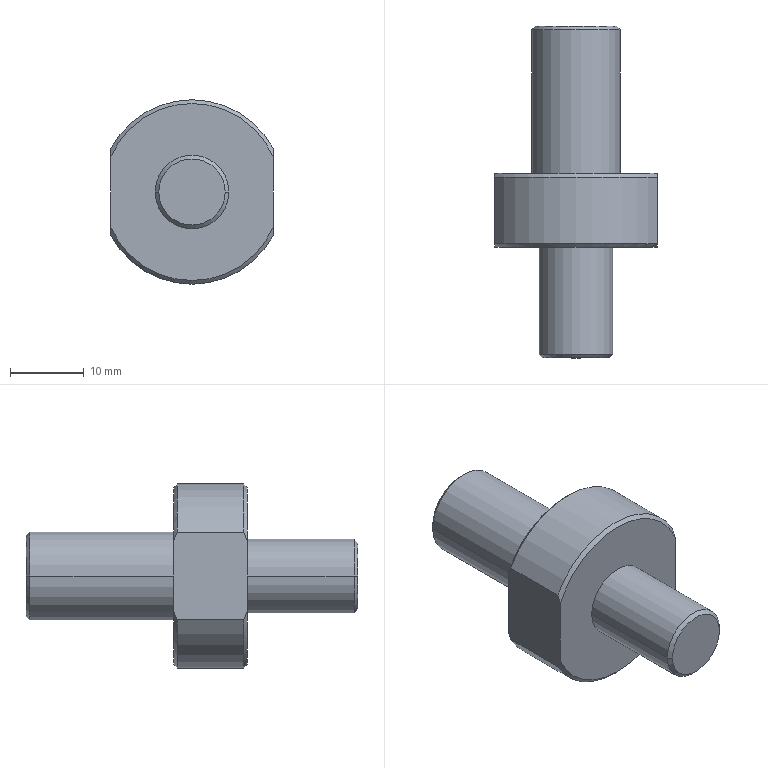Part | STEP file | Polisher lower hinge | 1 solid | 24 faces | box 22 x 45 x 25 mm | volume 7723 mm3 | cone 10 | cylinder 8 | plane 6 | commonest cylinder face diameters 5 x2 10 x2 12 x2 25 x2